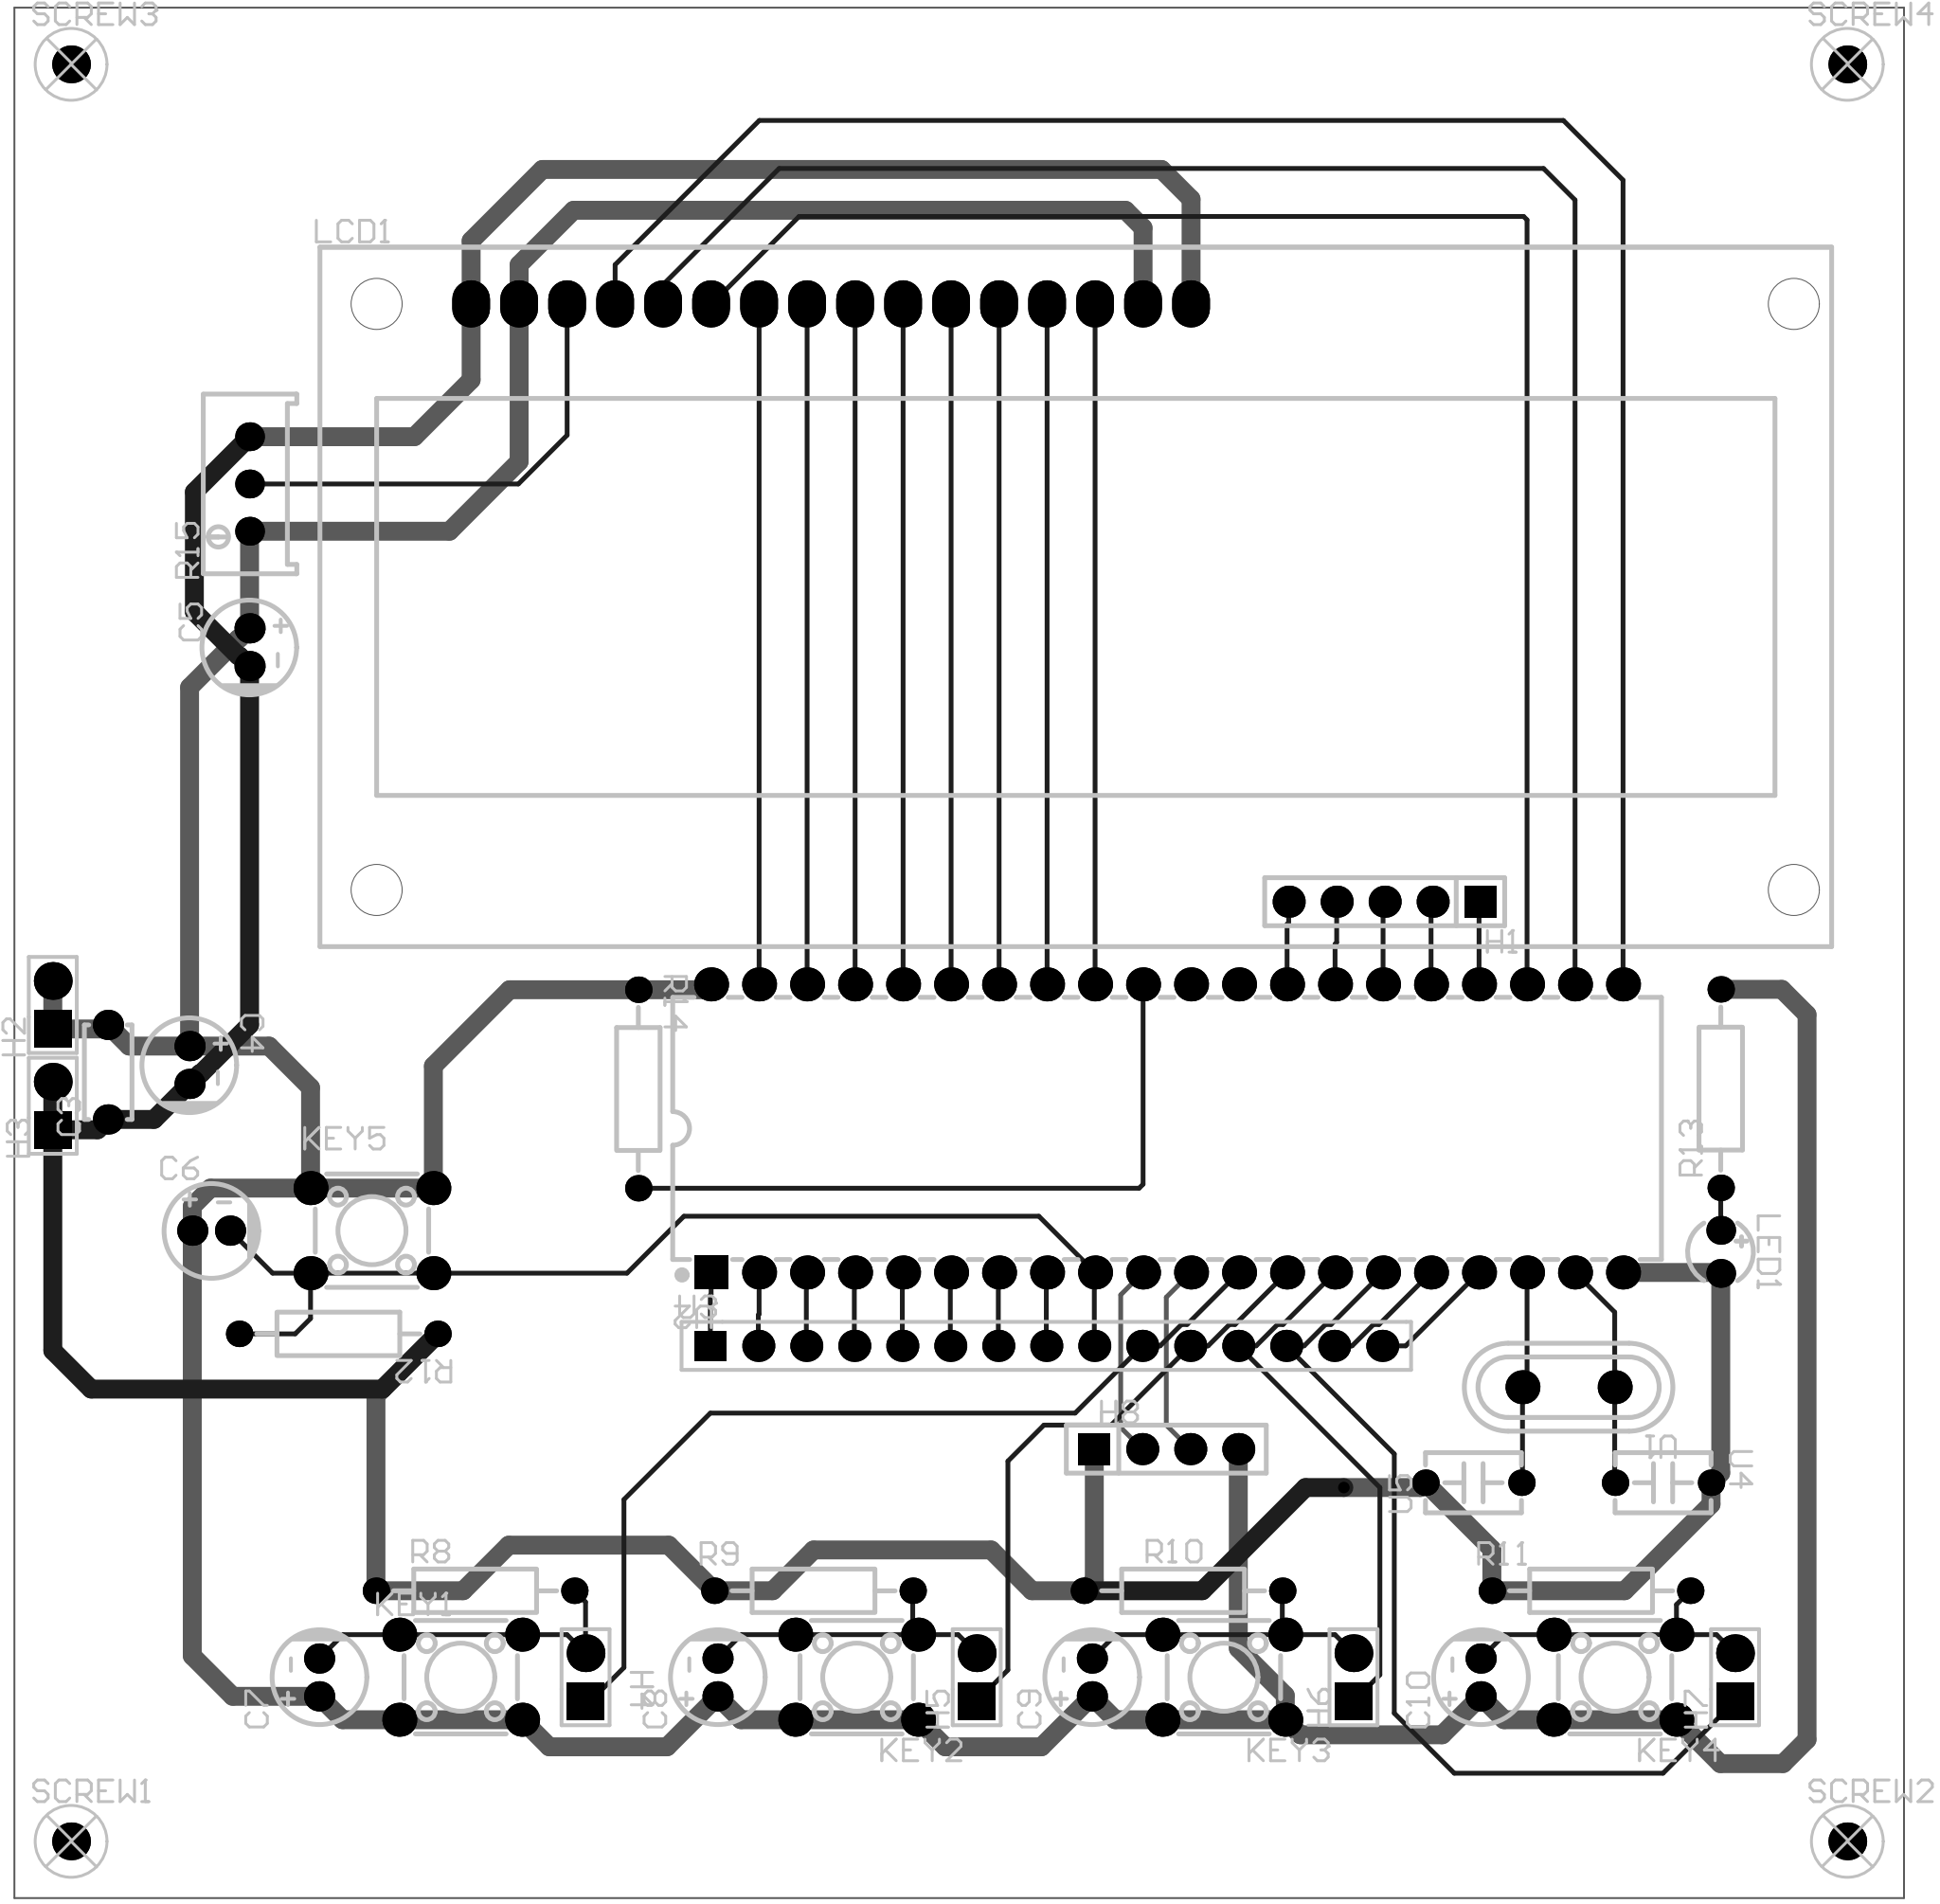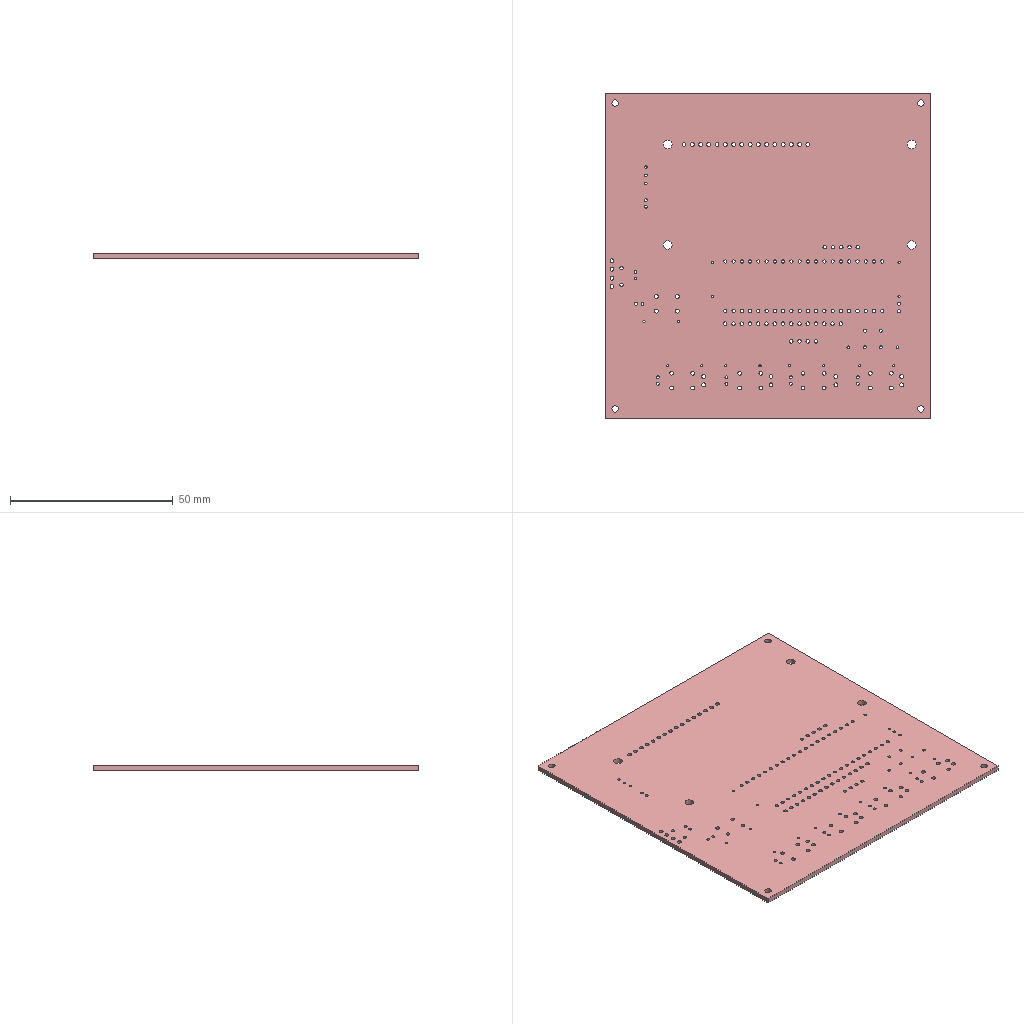Circuit board layout | Altium Designer | box 100 x 100 x 1.6 mm
Layer stack:
# Altium Designer layer stack of  (unit mm; dielectric type: 0 none, 1 core, 2 prepreg, 3 surface material)
index,name,kind,layer,copper_thickness_mm,dielectric_type,dielectric_thickness_mm,dielectric_material,dielectric_constant
0,Top Paste Mask Layer,other,,,,,,
1,Top Silkscreen Layer,other,,,,,,
2,Top Solder Mask Layer,dielectric,,,3,0.01,,3.3
3,Top Layer,copper,Top Layer,0.035,,,,
4,Dielectric1,dielectric,,,3,1.51,FR4,4.5
5,Bottom Layer,copper,Bottom Layer,0.035,,,,
6,Bottom Solder Mask Layer,dielectric,,,3,0.01,,3.3
7,Bottom Silkscreen Layer,other,,,,,,
8,Bottom Paste Mask Layer,other,,,,,,
# drill layer pairs: low layer,high layer
drill_pair,Top Layer,Bottom Layer
Part placement:
Designator,Comment,Layer,Footprint,Center-X(mm),Center-Y(mm),Rotation
C3,100nF,TopLayer,CAP-TH_L5.0-W2.5-P5.00-D1.0,81.153,119.888,90
C4,10uF,TopLayer,CAP-TH_BD5.0-P2.00-D0.5-FD-A,85.471,120.269,270
C5,10uF,TopLayer,CAP-TH_BD5.0-P2.00-D0.5-FD-A,88.646,142.367,270
C6,10uF,TopLayer,CAP-TH_BD5.0-P2.00-D0.5-FD-A,86.614,111.506,0
C7,10uF,TopLayer,CAP-TH_BD5.0-P2.00-D0.5-FD-A,92.329,87.871,90
C8,10uF,TopLayer,CAP-TH_BD5.0-P2.00-D0.5-FD-A,113.411,87.871,90
C9,10uF,TopLayer,CAP-TH_BD5.0-P2.00-D0.5-FD-A,133.223,87.871,90
C10,10uF,TopLayer,CAP-TH_BD5.0-P2.00-D0.5-FD-A,153.797,87.871,90
H1,PZ254V-11-05P,TopLayer,HDR-TH_5P-P2.54-V-M,148.717,128.905,180
H2,PZ254V-11-02P,TopLayer,HDR-TH_2P-P2.54-V-M,78.232,123.444,90
H3,PZ254V-11-02P,TopLayer,HDR-TH_2P-P2.54-V-M,78.232,118.11,90
H4,PZ254V-11-02P,TopLayer,HDR-TH_2P-P2.54-V-M,106.426,87.884,90
H5,PZ254V-11-02P,TopLayer,HDR-TH_2P-P2.54-V-M,127.127,87.884,90
H6,PZ254V-11-02P,TopLayer,HDR-TH_2P-P2.54-V-M,147.066,87.884,90
H7,PZ254V-11-02P,TopLayer,HDR-TH_2P-P2.54-V-M,167.259,87.884,90
LCD1,LCM1602K-NSW-BBW,TopLayer,MODULE-TH_LCM1602K,119.421,160.528,0
LED1,3A2RUD,TopLayer,LED-TH_BD3.5-P2.28_3A2RUC,166.502,110.384,270
SCREW1,,TopLayer,M2螺丝,79.2,79.2,0
SCREW2,,TopLayer,M2螺丝,173.2,79.2,0
SCREW3,,TopLayer,M2螺丝,79.2,173.2,0
SCREW4,,TopLayer,M2螺丝,173.2,173.2,0
U2,STC89C516RD+40I-PDIP40,TopLayer,DIP-40_L52.3-W13.9-P2.54-LS15.2-BL,137.201,116.913,0
U3,ZX-PM2.54-1-15PY,TopLayer,HDR-TH_15P-P2.54-V-F,130.81,105.41,0
U1,12MHz,TopLayer,HC-49S_L11.0-W4.7-P4.88,158.45,103.223,180
H8,,TopLayer,HDR-TH_4P-P2.54-V-F,137.16,99.949,0
KEY1,,TopLayer,SW-TH_4P-L6.0-W6.0-P4.50-LS6.5,99.822,87.884,180
KEY2,,TopLayer,SW-TH_4P-L6.0-W6.0-P4.50-LS6.5,120.777,87.884,180
KEY3,,TopLayer,SW-TH_4P-L6.0-W6.0-P4.50-LS6.5,140.208,87.884,180
KEY4,,TopLayer,SW-TH_4P-L6.0-W6.0-P4.50-LS6.5,160.909,87.884,180
R8,10kΩ,TopLayer,RES-TH_BD2.3-L6.5-P10.50-D0.5,100.584,92.456,0
R9,10kΩ,TopLayer,RES-TH_BD2.3-L6.5-P10.50-D0.5,118.491,92.456,0
R10,10kΩ,TopLayer,RES-TH_BD2.3-L6.5-P10.50-D0.5,138.049,92.456,0
R11,10kΩ,TopLayer,RES-TH_BD2.3-L6.5-P10.50-D0.5,159.639,92.456,0
R12,10kΩ,TopLayer,RES-TH_BD2.3-L6.5-P10.50-D0.5,93.345,106.045,180
R13,10kΩ,TopLayer,RES-TH_BD2.3-L6.5-P10.50-D0.5,166.502,119.02,90
R14,10kΩ,TopLayer,RES-TH_BD2.3-L6.5-P10.50-D0.5,109.22,118.999,270
U4,33pF,TopLayer,CAP-TH_L5.0-W2.5-P5.08-D0.7,163.449,98.171,180
U5,33pF,TopLayer,CAP-TH_L5.0-W2.5-P5.08-D0.7,153.416,98.171,0
KEY5,,TopLayer,SW-TH_4P-L6.0-W6.0-P4.50-LS6.5,95.123,111.506,180
R15,10kΩ,TopLayer,RES-ADJ-TH_3P-L10.0-W10.0-P2.50-L,88.646,151.003,90
Pad and via stacks:
# Altium Designer via and pad stacks of  (unit mm). Each distinct definition once, with the count of objects using it.
# via: kind,start_layer,end_layer,hole_mm,diameter_mm,mode(0 simple;1 top-mid-bottom;2 full stack),diameter_per_layer,count,example_net
# pad: kind,layer,hole_mm,hole_type(0 round;1 square;2 slot),plating,top_size,top_shape(1 round;2 rect;3 octagon;9 rounded rect),mid_size,bottom_size,mode,footprint,size_per_layer,count,example
pad,Multi-Layer,1,0,plated,1.6x1.6,1,1.6x1.6,1.6x1.6,0,CAP-TH_L5.0-W2.5-P5.00-D1.0,,2,C3.1
pad,Multi-Layer,0.9,0,plated,1.6x1.6,1,1.6x1.6,1.6x1.6,0,CAP-TH_BD5.0-P2.00-D0.5-FD-A,,14,C4.2
pad,Multi-Layer,1.1,0,plated,1.7x1.7,2,1.7x1.7,1.7x1.7,0,HDR-TH_5P-P2.54-V-M,,1,H1.1
pad,Multi-Layer,1.1,0,plated,1.7x1.7,1,1.7x1.7,1.7x1.7,0,HDR-TH_5P-P2.54-V-M,,4,H1.2
pad,Multi-Layer,1.2,0,plated,2x2,2,2x2,2x2,0,HDR-TH_2P-P2.54-V-M,,6,H2.1
pad,Multi-Layer,1.2,0,plated,2x2,1,2x2,2x2,0,HDR-TH_2P-P2.54-V-M,,6,H2.2
pad,Multi-Layer,1.2,0,plated,2.5x2,1,2.5x2,2.5x2,0,MODULE-TH_LCM1602K,,16,LCD1.1
pad,Multi-Layer,0.9144,0,plated,1.524x1.524,1,1.524x1.524,1.524x1.524,0,LED-TH_BD3.5-P2.28_3A2RUC,,2,LED1.2
pad,Multi-Layer,2,0,plated,2x2,1,2x2,2x2,0,M2\u00C2\u00DD\u00CB\u00BF,,4,SCREW1.1
pad,Multi-Layer,1,0,plated,1.8x1.8,1,1.8x1.8,1.8x1.8,0,DIP-40_L52.3-W13.9-P2.54-LS15.2-BL,,39,U2.19
pad,Multi-Layer,1,0,plated,1.8x1.8,2,1.8x1.8,1.8x1.8,0,DIP-40_L52.3-W13.9-P2.54-LS15.2-BL,,1,U2.1
pad,Multi-Layer,1.1,0,plated,1.7x1.7,1,1.7x1.7,1.7x1.7,0,HDR-TH_15P-P2.54-V-F,,14,U3.15
pad,Multi-Layer,1.1,0,plated,1.7x1.575,2,1.7x1.575,1.7x1.575,0,HDR-TH_15P-P2.54-V-F,,1,U3.1
pad,Multi-Layer,0.9,0,plated,1.8x1.8,1,1.8x1.8,1.8x1.8,0,HC-49S_L11.0-W4.7-P4.88,,2,U1.1
pad,Multi-Layer,1.1,0,plated,1.7x1.7,2,1.7x1.7,1.7x1.7,0,HDR-TH_4P-P2.54-V-F,,1,H8.1
pad,Multi-Layer,1.1,0,plated,1.7x1.7,1,1.7x1.7,1.7x1.7,0,HDR-TH_4P-P2.54-V-F,,3,H8.2
pad,Multi-Layer,1.2,0,plated,1.8x1.8,1,1.8x1.8,1.8x1.8,0,SW-TH_4P-L6.0-W6.0-P4.50-LS6.5,,20,KEY1.1
pad,Multi-Layer,0.7,0,plated,1.4x1.4,1,1.4x1.4,1.4x1.4,0,RES-TH_BD2.3-L6.5-P10.50-D0.5,,14,R8.1
pad,Multi-Layer,0.8,0,plated,1.4x1.4,1,1.4x1.4,1.4x1.4,0,CAP-TH_L5.0-W2.5-P5.08-D0.7,,4,U4.1
pad,Multi-Layer,0.762,0,plated,1.524x1.524,1,1.524x1.524,1.524x1.524,0,RES-ADJ-TH_3P-L10.0-W10.0-P2.50-L,,3,R15.2
via,Top Layer,Bottom Layer,0.3048,0.61,0,,1,GND